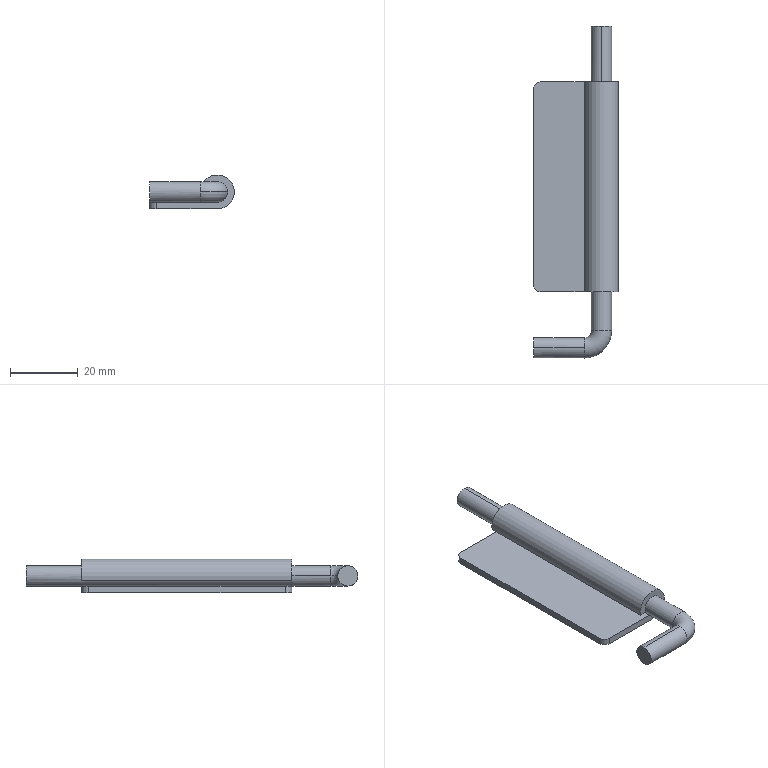Part | SolidWorks | features Extrusion 1, Fillet 1, Sweep 1 | 1 solid | 19 faces | box 25 x 98 x 10 mm | volume 8135 mm3 | cylinder 9 | plane 8 | torus 2 | commonest cylinder face diameters 6 x6 4 x2 10 x1
STEP:
#1=CARTESIAN_POINT('',(-5.,-19.5,0.));
#2=VERTEX_POINT('',#1);
#3=CARTESIAN_POINT('',(-5.,-16.5,3.));
#4=VERTEX_POINT('',#3);
#5=CARTESIAN_POINT('',(-5.,-16.5,0.));
#6=DIRECTION('',(-1.,0.,0.));
#7=DIRECTION('',(0.,0.,-1.));
#8=AXIS2_PLACEMENT_3D('',#5,#6,#7);
#9=CIRCLE('',#8,3.);
#10=EDGE_CURVE('',#2,#4,#9,.T.);
#11=ORIENTED_EDGE('',*,*,#10,.F.);
#12=CARTESIAN_POINT('',(3.,-11.5,0.));
#13=VERTEX_POINT('',#12);
#14=CARTESIAN_POINT('',(-5.,-11.5,0.));
#15=DIRECTION('',(0.,0.,1.));
#16=DIRECTION('',(1.,0.,0.));
#17=AXIS2_PLACEMENT_3D('',#14,#15,#16);
#18=CIRCLE('',#17,8.);
#19=EDGE_CURVE('',#2,#13,#18,.T.);
#20=ORIENTED_EDGE('',*,*,#19,.T.);
#21=CARTESIAN_POINT('',(-3.,-11.5,0.));
#22=VERTEX_POINT('',#21);
#23=CARTESIAN_POINT('',(0.,-11.5,0.));
#24=DIRECTION('',(0.,-1.,0.));
#25=DIRECTION('',(0.,0.,-1.));
#26=AXIS2_PLACEMENT_3D('',#23,#24,#25);
#27=CIRCLE('',#26,3.);
#28=EDGE_CURVE('',#13,#22,#27,.T.);
#29=ORIENTED_EDGE('',*,*,#28,.T.);
#30=CARTESIAN_POINT('',(-5.,-13.5,0.));
#31=VERTEX_POINT('',#30);
#32=CARTESIAN_POINT('',(-5.,-11.5,0.));
#33=DIRECTION('',(0.,0.,1.));
#34=DIRECTION('',(1.,0.,0.));
#35=AXIS2_PLACEMENT_3D('',#32,#33,#34);
#36=CIRCLE('',#35,2.);
#37=EDGE_CURVE('',#31,#22,#36,.T.);
#38=ORIENTED_EDGE('',*,*,#37,.F.);
#39=CARTESIAN_POINT('',(-5.,-16.5,0.));
#40=DIRECTION('',(-1.,0.,0.));
#41=DIRECTION('',(0.,0.,-1.));
#42=AXIS2_PLACEMENT_3D('',#39,#40,#41);
#43=CIRCLE('',#42,3.);
#44=EDGE_CURVE('',#4,#31,#43,.T.);
#45=ORIENTED_EDGE('',*,*,#44,.F.);
#46=EDGE_LOOP('',(#11,#20,#29,#38,#45));
#47=FACE_OUTER_BOUND('',#46,.T.);
#48=CARTESIAN_POINT('',(-5.,-11.5,0.));
#49=DIRECTION('',(0.,0.,1.));
#50=DIRECTION('',(1.,0.,0.));
#51=AXIS2_PLACEMENT_3D('',#48,#49,#50);
#52=TOROIDAL_SURFACE('',#51,5.,3.);
#53=ADVANCED_FACE('',(#47),#52,.T.);
#54=ORIENTED_EDGE('',*,*,#28,.F.);
#55=CARTESIAN_POINT('',(3.,0.,0.));
#56=VERTEX_POINT('',#55);
#57=CARTESIAN_POINT('',(3.,-11.5,0.));
#58=DIRECTION('',(0.,1.,0.));
#59=VECTOR('',#58,1000.);
#60=LINE('',#57,#59);
#61=EDGE_CURVE('',#13,#56,#60,.T.);
#62=ORIENTED_EDGE('',*,*,#61,.T.);
#63=CARTESIAN_POINT('',(-3.,0.,0.));
#64=VERTEX_POINT('',#63);
#65=CARTESIAN_POINT('',(0.,0.,0.));
#66=DIRECTION('',(0.,-1.,0.));
#67=DIRECTION('',(0.,0.,1.));
#68=AXIS2_PLACEMENT_3D('',#65,#66,#67);
#69=CIRCLE('',#68,3.);
#70=EDGE_CURVE('',#56,#64,#69,.T.);
#71=ORIENTED_EDGE('',*,*,#70,.T.);
#72=CARTESIAN_POINT('',(-3.,-11.5,0.));
#73=DIRECTION('',(0.,1.,0.));
#74=VECTOR('',#73,1000.);
#75=LINE('',#72,#74);
#76=EDGE_CURVE('',#22,#64,#75,.T.);
#77=ORIENTED_EDGE('',*,*,#76,.F.);
#78=EDGE_LOOP('',(#54,#62,#71,#77));
#79=FACE_OUTER_BOUND('',#78,.T.);
#80=CARTESIAN_POINT('',(0.,-11.5,0.));
#81=DIRECTION('',(0.,1.,0.));
#82=DIRECTION('',(-1.,0.,0.));
#83=AXIS2_PLACEMENT_3D('',#80,#81,#82);
#84=CYLINDRICAL_SURFACE('',#83,3.);
#85=ADVANCED_FACE('',(#79),#84,.T.);
#86=CARTESIAN_POINT('',(-20.,-16.5,3.));
#87=VERTEX_POINT('',#86);
#88=CARTESIAN_POINT('',(-20.,-16.5,-3.));
#89=VERTEX_POINT('',#88);
#90=CARTESIAN_POINT('',(-20.,-16.5,0.));
#91=DIRECTION('',(-1.,0.,0.));
#92=DIRECTION('',(0.,0.,-1.));
#93=AXIS2_PLACEMENT_3D('',#90,#91,#92);
#94=CIRCLE('',#93,3.);
#95=EDGE_CURVE('',#87,#89,#94,.T.);
#96=ORIENTED_EDGE('',*,*,#95,.F.);
#97=CARTESIAN_POINT('',(-20.,-16.5,3.));
#98=DIRECTION('',(1.,0.,0.));
#99=VECTOR('',#98,1000.);
#100=LINE('',#97,#99);
#101=EDGE_CURVE('',#87,#4,#100,.T.);
#102=ORIENTED_EDGE('',*,*,#101,.T.);
#103=ORIENTED_EDGE('',*,*,#44,.T.);
#104=CARTESIAN_POINT('',(-5.,-16.5,-3.));
#105=VERTEX_POINT('',#104);
#106=CARTESIAN_POINT('',(-5.,-16.5,0.));
#107=DIRECTION('',(-1.,0.,0.));
#108=DIRECTION('',(0.,0.,-1.));
#109=AXIS2_PLACEMENT_3D('',#106,#107,#108);
#110=CIRCLE('',#109,3.);
#111=EDGE_CURVE('',#31,#105,#110,.T.);
#112=ORIENTED_EDGE('',*,*,#111,.T.);
#113=CARTESIAN_POINT('',(-20.,-16.5,-3.));
#114=DIRECTION('',(1.,0.,0.));
#115=VECTOR('',#114,1000.);
#116=LINE('',#113,#115);
#117=EDGE_CURVE('',#89,#105,#116,.T.);
#118=ORIENTED_EDGE('',*,*,#117,.F.);
#119=EDGE_LOOP('',(#96,#102,#103,#112,#118));
#120=FACE_OUTER_BOUND('',#119,.T.);
#121=CARTESIAN_POINT('',(-20.,-16.5,0.));
#122=DIRECTION('',(1.,0.,0.));
#123=DIRECTION('',(0.,0.,-1.));
#124=AXIS2_PLACEMENT_3D('',#121,#122,#123);
#125=CYLINDRICAL_SURFACE('',#124,3.);
#126=ADVANCED_FACE('',(#120),#125,.T.);
#127=CARTESIAN_POINT('',(0.,62.,-3.));
#128=VERTEX_POINT('',#127);
#129=CARTESIAN_POINT('',(0.,62.,3.));
#130=VERTEX_POINT('',#129);
#131=CARTESIAN_POINT('',(0.,62.,0.));
#132=DIRECTION('',(0.,-1.,0.));
#133=DIRECTION('',(0.,0.,1.));
#134=AXIS2_PLACEMENT_3D('',#131,#132,#133);
#135=CIRCLE('',#134,3.);
#136=EDGE_CURVE('',#128,#130,#135,.T.);
#137=ORIENTED_EDGE('',*,*,#136,.F.);
#138=CARTESIAN_POINT('',(0.,78.5,-3.));
#139=VERTEX_POINT('',#138);
#140=CARTESIAN_POINT('',(0.,0.,-3.));
#141=DIRECTION('',(0.,1.,0.));
#142=VECTOR('',#141,1000.);
#143=LINE('',#140,#142);
#144=EDGE_CURVE('',#128,#139,#143,.T.);
#145=ORIENTED_EDGE('',*,*,#144,.T.);
#146=CARTESIAN_POINT('',(0.,78.5,3.));
#147=VERTEX_POINT('',#146);
#148=CARTESIAN_POINT('',(0.,78.5,0.));
#149=DIRECTION('',(0.,-1.,0.));
#150=DIRECTION('',(0.,0.,-1.));
#151=AXIS2_PLACEMENT_3D('',#148,#149,#150);
#152=CIRCLE('',#151,3.);
#153=EDGE_CURVE('',#139,#147,#152,.T.);
#154=ORIENTED_EDGE('',*,*,#153,.T.);
#155=CARTESIAN_POINT('',(0.,0.,3.));
#156=DIRECTION('',(0.,1.,0.));
#157=VECTOR('',#156,1000.);
#158=LINE('',#155,#157);
#159=EDGE_CURVE('',#130,#147,#158,.T.);
#160=ORIENTED_EDGE('',*,*,#159,.F.);
#161=EDGE_LOOP('',(#137,#145,#154,#160));
#162=FACE_OUTER_BOUND('',#161,.T.);
#163=CARTESIAN_POINT('',(0.,0.,0.));
#164=DIRECTION('',(0.,1.,0.));
#165=DIRECTION('',(0.,0.,1.));
#166=AXIS2_PLACEMENT_3D('',#163,#164,#165);
#167=CYLINDRICAL_SURFACE('',#166,3.);
#168=ADVANCED_FACE('',(#162),#167,.T.);
#169=CARTESIAN_POINT('',(-4.83,0.,-1.294));
#170=VERTEX_POINT('',#169);
#171=CARTESIAN_POINT('',(0.,0.,-5.));
#172=VERTEX_POINT('',#171);
#173=CARTESIAN_POINT('',(0.,0.,0.));
#174=DIRECTION('',(0.,1.,0.));
#175=DIRECTION('',(0.,0.,1.));
#176=AXIS2_PLACEMENT_3D('',#173,#174,#175);
#177=CIRCLE('',#176,5.);
#178=EDGE_CURVE('',#170,#172,#177,.T.);
#179=ORIENTED_EDGE('',*,*,#178,.T.);
#180=CARTESIAN_POINT('',(0.,62.,-5.));
#181=VERTEX_POINT('',#180);
#182=CARTESIAN_POINT('',(0.,62.,-5.));
#183=DIRECTION('',(0.,-1.,0.));
#184=VECTOR('',#183,1000.);
#185=LINE('',#182,#184);
#186=EDGE_CURVE('',#181,#172,#185,.T.);
#187=ORIENTED_EDGE('',*,*,#186,.F.);
#188=CARTESIAN_POINT('',(-4.83,62.,-1.294));
#189=VERTEX_POINT('',#188);
#190=CARTESIAN_POINT('',(0.,62.,0.));
#191=DIRECTION('',(0.,1.,0.));
#192=DIRECTION('',(0.,0.,1.));
#193=AXIS2_PLACEMENT_3D('',#190,#191,#192);
#194=CIRCLE('',#193,5.);
#195=EDGE_CURVE('',#189,#181,#194,.T.);
#196=ORIENTED_EDGE('',*,*,#195,.F.);
#197=CARTESIAN_POINT('',(-4.83,62.,-1.294));
#198=DIRECTION('',(0.,-1.,0.));
#199=VECTOR('',#198,1000.);
#200=LINE('',#197,#199);
#201=EDGE_CURVE('',#189,#170,#200,.T.);
#202=ORIENTED_EDGE('',*,*,#201,.T.);
#203=EDGE_LOOP('',(#179,#187,#196,#202));
#204=FACE_OUTER_BOUND('',#203,.T.);
#205=CARTESIAN_POINT('',(0.,62.,0.));
#206=DIRECTION('',(0.,-1.,0.));
#207=DIRECTION('',(0.,0.,-1.));
#208=AXIS2_PLACEMENT_3D('',#205,#206,#207);
#209=CYLINDRICAL_SURFACE('',#208,5.);
#210=ADVANCED_FACE('',(#204),#209,.T.);
#211=CARTESIAN_POINT('',(-18.,0.,-5.));
#212=VERTEX_POINT('',#211);
#213=CARTESIAN_POINT('',(0.,0.,-5.));
#214=DIRECTION('',(-1.,0.,0.));
#215=VECTOR('',#214,1000.);
#216=LINE('',#213,#215);
#217=EDGE_CURVE('',#172,#212,#216,.T.);
#218=ORIENTED_EDGE('',*,*,#217,.T.);
#219=CARTESIAN_POINT('',(-20.,2.,-5.));
#220=VERTEX_POINT('',#219);
#221=CARTESIAN_POINT('',(-18.,2.,-5.));
#222=DIRECTION('',(0.,0.,-1.));
#223=DIRECTION('',(1.,0.,0.));
#224=AXIS2_PLACEMENT_3D('',#221,#222,#223);
#225=CIRCLE('',#224,2.);
#226=EDGE_CURVE('',#212,#220,#225,.T.);
#227=ORIENTED_EDGE('',*,*,#226,.T.);
#228=CARTESIAN_POINT('',(-20.,60.,-5.));
#229=VERTEX_POINT('',#228);
#230=CARTESIAN_POINT('',(-20.,62.,-5.));
#231=DIRECTION('',(0.,-1.,0.));
#232=VECTOR('',#231,1000.);
#233=LINE('',#230,#232);
#234=EDGE_CURVE('',#229,#220,#233,.T.);
#235=ORIENTED_EDGE('',*,*,#234,.F.);
#236=CARTESIAN_POINT('',(-18.,62.,-5.));
#237=VERTEX_POINT('',#236);
#238=CARTESIAN_POINT('',(-18.,60.,-5.));
#239=DIRECTION('',(0.,0.,-1.));
#240=DIRECTION('',(1.,0.,0.));
#241=AXIS2_PLACEMENT_3D('',#238,#239,#240);
#242=CIRCLE('',#241,2.);
#243=EDGE_CURVE('',#229,#237,#242,.T.);
#244=ORIENTED_EDGE('',*,*,#243,.T.);
#245=CARTESIAN_POINT('',(0.,62.,-5.));
#246=DIRECTION('',(-1.,0.,0.));
#247=VECTOR('',#246,1000.);
#248=LINE('',#245,#247);
#249=EDGE_CURVE('',#181,#237,#248,.T.);
#250=ORIENTED_EDGE('',*,*,#249,.F.);
#251=ORIENTED_EDGE('',*,*,#186,.T.);
#252=EDGE_LOOP('',(#218,#227,#235,#244,#250,#251));
#253=FACE_OUTER_BOUND('',#252,.T.);
#254=CARTESIAN_POINT('',(0.,62.,-5.));
#255=DIRECTION('',(0.,0.,1.));
#256=DIRECTION('',(1.,0.,0.));
#257=AXIS2_PLACEMENT_3D('',#254,#255,#256);
#258=PLANE('',#257);
#259=ADVANCED_FACE('',(#253),#258,.F.);
#260=ORIENTED_EDGE('',*,*,#234,.T.);
#261=CARTESIAN_POINT('',(-20.,2.,-3.));
#262=VERTEX_POINT('',#261);
#263=CARTESIAN_POINT('',(-20.,2.,-3.));
#264=DIRECTION('',(0.,0.,1.));
#265=VECTOR('',#264,1000.);
#266=LINE('',#263,#265);
#267=EDGE_CURVE('',#220,#262,#266,.T.);
#268=ORIENTED_EDGE('',*,*,#267,.T.);
#269=CARTESIAN_POINT('',(-20.,60.,-3.));
#270=VERTEX_POINT('',#269);
#271=CARTESIAN_POINT('',(-20.,62.,-3.));
#272=DIRECTION('',(0.,-1.,0.));
#273=VECTOR('',#272,1000.);
#274=LINE('',#271,#273);
#275=EDGE_CURVE('',#270,#262,#274,.T.);
#276=ORIENTED_EDGE('',*,*,#275,.F.);
#277=CARTESIAN_POINT('',(-20.,60.,-5.));
#278=DIRECTION('',(0.,0.,-1.));
#279=VECTOR('',#278,1000.);
#280=LINE('',#277,#279);
#281=EDGE_CURVE('',#270,#229,#280,.T.);
#282=ORIENTED_EDGE('',*,*,#281,.T.);
#283=EDGE_LOOP('',(#260,#268,#276,#282));
#284=FACE_OUTER_BOUND('',#283,.T.);
#285=CARTESIAN_POINT('',(-20.,62.,-3.));
#286=DIRECTION('',(1.,0.,0.));
#287=DIRECTION('',(0.,0.,-1.));
#288=AXIS2_PLACEMENT_3D('',#285,#286,#287);
#289=PLANE('',#288);
#290=ADVANCED_FACE('',(#284),#289,.F.);
#291=ORIENTED_EDGE('',*,*,#275,.T.);
#292=CARTESIAN_POINT('',(-18.,0.,-3.));
#293=VERTEX_POINT('',#292);
#294=CARTESIAN_POINT('',(-18.,2.,-3.));
#295=DIRECTION('',(0.,0.,1.));
#296=DIRECTION('',(-1.,0.,0.));
#297=AXIS2_PLACEMENT_3D('',#294,#295,#296);
#298=CIRCLE('',#297,2.);
#299=EDGE_CURVE('',#262,#293,#298,.T.);
#300=ORIENTED_EDGE('',*,*,#299,.T.);
#301=CARTESIAN_POINT('',(0.,0.,-3.));
#302=VERTEX_POINT('',#301);
#303=CARTESIAN_POINT('',(0.,0.,-3.));
#304=DIRECTION('',(1.,0.,0.));
#305=VECTOR('',#304,1000.);
#306=LINE('',#303,#305);
#307=EDGE_CURVE('',#293,#302,#306,.T.);
#308=ORIENTED_EDGE('',*,*,#307,.T.);
#309=CARTESIAN_POINT('',(0.,62.,-3.));
#310=DIRECTION('',(0.,-1.,0.));
#311=VECTOR('',#310,1000.);
#312=LINE('',#309,#311);
#313=EDGE_CURVE('',#128,#302,#312,.T.);
#314=ORIENTED_EDGE('',*,*,#313,.F.);
#315=CARTESIAN_POINT('',(-18.,62.,-3.));
#316=VERTEX_POINT('',#315);
#317=CARTESIAN_POINT('',(0.,62.,-3.));
#318=DIRECTION('',(1.,0.,0.));
#319=VECTOR('',#318,1000.);
#320=LINE('',#317,#319);
#321=EDGE_CURVE('',#316,#128,#320,.T.);
#322=ORIENTED_EDGE('',*,*,#321,.F.);
#323=CARTESIAN_POINT('',(-18.,60.,-3.));
#324=DIRECTION('',(0.,0.,1.));
#325=DIRECTION('',(-1.,0.,0.));
#326=AXIS2_PLACEMENT_3D('',#323,#324,#325);
#327=CIRCLE('',#326,2.);
#328=EDGE_CURVE('',#316,#270,#327,.T.);
#329=ORIENTED_EDGE('',*,*,#328,.T.);
#330=EDGE_LOOP('',(#291,#300,#308,#314,#322,#329));
#331=FACE_OUTER_BOUND('',#330,.T.);
#332=CARTESIAN_POINT('',(0.,62.,-3.));
#333=DIRECTION('',(0.,0.,-1.));
#334=DIRECTION('',(-1.,0.,0.));
#335=AXIS2_PLACEMENT_3D('',#332,#333,#334);
#336=PLANE('',#335);
#337=ADVANCED_FACE('',(#331),#336,.F.);
#338=CARTESIAN_POINT('',(-2.898,0.,-0.7765));
#339=VERTEX_POINT('',#338);
#340=CARTESIAN_POINT('',(-4.83,0.,-1.294));
#341=DIRECTION('',(-0.9659,0.,-0.2588));
#342=VECTOR('',#341,1000.);
#343=LINE('',#340,#342);
#344=EDGE_CURVE('',#339,#170,#343,.T.);
#345=ORIENTED_EDGE('',*,*,#344,.T.);
#346=ORIENTED_EDGE('',*,*,#201,.F.);
#347=CARTESIAN_POINT('',(-2.898,62.,-0.7765));
#348=VERTEX_POINT('',#347);
#349=CARTESIAN_POINT('',(-4.83,62.,-1.294));
#350=DIRECTION('',(-0.9659,0.,-0.2588));
#351=VECTOR('',#350,1000.);
#352=LINE('',#349,#351);
#353=EDGE_CURVE('',#348,#189,#352,.T.);
#354=ORIENTED_EDGE('',*,*,#353,.F.);
#355=CARTESIAN_POINT('',(-2.898,62.,-0.7765));
#356=DIRECTION('',(0.,-1.,0.));
#357=VECTOR('',#356,1000.);
#358=LINE('',#355,#357);
#359=EDGE_CURVE('',#348,#339,#358,.T.);
#360=ORIENTED_EDGE('',*,*,#359,.T.);
#361=EDGE_LOOP('',(#345,#346,#354,#360));
#362=FACE_OUTER_BOUND('',#361,.T.);
#363=CARTESIAN_POINT('',(-4.83,62.,-1.294));
#364=DIRECTION('',(-0.2588,0.,0.9659));
#365=DIRECTION('',(0.9659,0.,0.2588));
#366=AXIS2_PLACEMENT_3D('',#363,#364,#365);
#367=PLANE('',#366);
#368=ADVANCED_FACE('',(#362),#367,.F.);
#369=ORIENTED_EDGE('',*,*,#249,.T.);
#370=CARTESIAN_POINT('',(-18.,62.,-3.));
#371=DIRECTION('',(0.,0.,1.));
#372=VECTOR('',#371,1000.);
#373=LINE('',#370,#372);
#374=EDGE_CURVE('',#237,#316,#373,.T.);
#375=ORIENTED_EDGE('',*,*,#374,.T.);
#376=ORIENTED_EDGE('',*,*,#321,.T.);
#377=ORIENTED_EDGE('',*,*,#136,.T.);
#378=CARTESIAN_POINT('',(0.,62.,0.));
#379=DIRECTION('',(0.,-1.,0.));
#380=DIRECTION('',(0.,0.,1.));
#381=AXIS2_PLACEMENT_3D('',#378,#379,#380);
#382=CIRCLE('',#381,3.);
#383=EDGE_CURVE('',#130,#348,#382,.T.);
#384=ORIENTED_EDGE('',*,*,#383,.T.);
#385=ORIENTED_EDGE('',*,*,#353,.T.);
#386=ORIENTED_EDGE('',*,*,#195,.T.);
#387=EDGE_LOOP('',(#369,#375,#376,#377,#384,#385,#386));
#388=FACE_OUTER_BOUND('',#387,.T.);
#389=CARTESIAN_POINT('',(0.,62.,0.));
#390=DIRECTION('',(0.,1.,0.));
#391=DIRECTION('',(0.,0.,1.));
#392=AXIS2_PLACEMENT_3D('',#389,#390,#391);
#393=PLANE('',#392);
#394=ADVANCED_FACE('',(#388),#393,.T.);
#395=ORIENTED_EDGE('',*,*,#307,.F.);
#396=CARTESIAN_POINT('',(-18.,0.,0.));
#397=DIRECTION('',(0.,0.,-1.));
#398=VECTOR('',#397,1000.);
#399=LINE('',#396,#398);
#400=EDGE_CURVE('',#293,#212,#399,.T.);
#401=ORIENTED_EDGE('',*,*,#400,.T.);
#402=ORIENTED_EDGE('',*,*,#217,.F.);
#403=ORIENTED_EDGE('',*,*,#178,.F.);
#404=ORIENTED_EDGE('',*,*,#344,.F.);
#405=CARTESIAN_POINT('',(0.,0.,0.));
#406=DIRECTION('',(0.,-1.,0.));
#407=DIRECTION('',(0.,0.,1.));
#408=AXIS2_PLACEMENT_3D('',#405,#406,#407);
#409=CIRCLE('',#408,3.);
#410=EDGE_CURVE('',#64,#339,#409,.T.);
#411=ORIENTED_EDGE('',*,*,#410,.F.);
#412=ORIENTED_EDGE('',*,*,#70,.F.);
#413=CARTESIAN_POINT('',(0.,0.,0.));
#414=DIRECTION('',(0.,-1.,0.));
#415=DIRECTION('',(0.,0.,1.));
#416=AXIS2_PLACEMENT_3D('',#413,#414,#415);
#417=CIRCLE('',#416,3.);
#418=EDGE_CURVE('',#302,#56,#417,.T.);
#419=ORIENTED_EDGE('',*,*,#418,.F.);
#420=EDGE_LOOP('',(#395,#401,#402,#403,#404,#411,#412,#419));
#421=FACE_OUTER_BOUND('',#420,.T.);
#422=CARTESIAN_POINT('',(0.,0.,0.));
#423=DIRECTION('',(0.,1.,0.));
#424=DIRECTION('',(0.,0.,1.));
#425=AXIS2_PLACEMENT_3D('',#422,#423,#424);
#426=PLANE('',#425);
#427=ADVANCED_FACE('',(#421),#426,.F.);
#428=ORIENTED_EDGE('',*,*,#144,.F.);
#429=ORIENTED_EDGE('',*,*,#313,.T.);
#430=CARTESIAN_POINT('',(0.,0.,0.));
#431=DIRECTION('',(0.,-1.,0.));
#432=DIRECTION('',(0.,0.,-1.));
#433=AXIS2_PLACEMENT_3D('',#430,#431,#432);
#434=CIRCLE('',#433,3.);
#435=EDGE_CURVE('',#339,#302,#434,.T.);
#436=ORIENTED_EDGE('',*,*,#435,.F.);
#437=ORIENTED_EDGE('',*,*,#359,.F.);
#438=ORIENTED_EDGE('',*,*,#383,.F.);
#439=ORIENTED_EDGE('',*,*,#159,.T.);
#440=CARTESIAN_POINT('',(0.,78.5,0.));
#441=DIRECTION('',(0.,-1.,0.));
#442=DIRECTION('',(0.,0.,-1.));
#443=AXIS2_PLACEMENT_3D('',#440,#441,#442);
#444=CIRCLE('',#443,3.);
#445=EDGE_CURVE('',#147,#139,#444,.T.);
#446=ORIENTED_EDGE('',*,*,#445,.T.);
#447=EDGE_LOOP('',(#428,#429,#436,#437,#438,#439,#446));
#448=FACE_OUTER_BOUND('',#447,.T.);
#449=CARTESIAN_POINT('',(0.,0.,0.));
#450=DIRECTION('',(0.,1.,0.));
#451=DIRECTION('',(0.,0.,1.));
#452=AXIS2_PLACEMENT_3D('',#449,#450,#451);
#453=CYLINDRICAL_SURFACE('',#452,3.);
#454=ADVANCED_FACE('',(#448),#453,.T.);
#455=ORIENTED_EDGE('',*,*,#61,.F.);
#456=CARTESIAN_POINT('',(0.,-11.5,0.));
#457=DIRECTION('',(0.,-1.,0.));
#458=DIRECTION('',(0.,0.,-1.));
#459=AXIS2_PLACEMENT_3D('',#456,#457,#458);
#460=CIRCLE('',#459,3.);
#461=EDGE_CURVE('',#22,#13,#460,.T.);
#462=ORIENTED_EDGE('',*,*,#461,.F.);
#463=ORIENTED_EDGE('',*,*,#76,.T.);
#464=ORIENTED_EDGE('',*,*,#410,.T.);
#465=ORIENTED_EDGE('',*,*,#435,.T.);
#466=ORIENTED_EDGE('',*,*,#418,.T.);
#467=EDGE_LOOP('',(#455,#462,#463,#464,#465,#466));
#468=FACE_OUTER_BOUND('',#467,.T.);
#469=CARTESIAN_POINT('',(0.,-11.5,0.));
#470=DIRECTION('',(0.,1.,0.));
#471=DIRECTION('',(-1.,0.,0.));
#472=AXIS2_PLACEMENT_3D('',#469,#470,#471);
#473=CYLINDRICAL_SURFACE('',#472,3.);
#474=ADVANCED_FACE('',(#468),#473,.T.);
#475=ORIENTED_EDGE('',*,*,#19,.F.);
#476=CARTESIAN_POINT('',(-5.,-16.5,0.));
#477=DIRECTION('',(-1.,0.,0.));
#478=DIRECTION('',(0.,0.,-1.));
#479=AXIS2_PLACEMENT_3D('',#476,#477,#478);
#480=CIRCLE('',#479,3.);
#481=EDGE_CURVE('',#105,#2,#480,.T.);
#482=ORIENTED_EDGE('',*,*,#481,.F.);
#483=ORIENTED_EDGE('',*,*,#111,.F.);
#484=ORIENTED_EDGE('',*,*,#37,.T.);
#485=ORIENTED_EDGE('',*,*,#461,.T.);
#486=EDGE_LOOP('',(#475,#482,#483,#484,#485));
#487=FACE_OUTER_BOUND('',#486,.T.);
#488=CARTESIAN_POINT('',(-5.,-11.5,0.));
#489=DIRECTION('',(0.,0.,1.));
#490=DIRECTION('',(1.,0.,0.));
#491=AXIS2_PLACEMENT_3D('',#488,#489,#490);
#492=TOROIDAL_SURFACE('',#491,5.,3.);
#493=ADVANCED_FACE('',(#487),#492,.T.);
#494=ORIENTED_EDGE('',*,*,#101,.F.);
#495=CARTESIAN_POINT('',(-20.,-16.5,0.));
#496=DIRECTION('',(-1.,0.,0.));
#497=DIRECTION('',(0.,0.,-1.));
#498=AXIS2_PLACEMENT_3D('',#495,#496,#497);
#499=CIRCLE('',#498,3.);
#500=EDGE_CURVE('',#89,#87,#499,.T.);
#501=ORIENTED_EDGE('',*,*,#500,.F.);
#502=ORIENTED_EDGE('',*,*,#117,.T.);
#503=ORIENTED_EDGE('',*,*,#481,.T.);
#504=ORIENTED_EDGE('',*,*,#10,.T.);
#505=EDGE_LOOP('',(#494,#501,#502,#503,#504));
#506=FACE_OUTER_BOUND('',#505,.T.);
#507=CARTESIAN_POINT('',(-20.,-16.5,0.));
#508=DIRECTION('',(1.,0.,0.));
#509=DIRECTION('',(0.,0.,-1.));
#510=AXIS2_PLACEMENT_3D('',#507,#508,#509);
#511=CYLINDRICAL_SURFACE('',#510,3.);
#512=ADVANCED_FACE('',(#506),#511,.T.);
#513=ORIENTED_EDGE('',*,*,#445,.F.);
#514=ORIENTED_EDGE('',*,*,#153,.F.);
#515=EDGE_LOOP('',(#513,#514));
#516=FACE_OUTER_BOUND('',#515,.T.);
#517=CARTESIAN_POINT('',(0.,78.5,0.));
#518=DIRECTION('',(0.,-1.,0.));
#519=DIRECTION('',(0.,0.,-1.));
#520=AXIS2_PLACEMENT_3D('',#517,#518,#519);
#521=PLANE('',#520);
#522=ADVANCED_FACE('',(#516),#521,.F.);
#523=ORIENTED_EDGE('',*,*,#500,.T.);
#524=ORIENTED_EDGE('',*,*,#95,.T.);
#525=EDGE_LOOP('',(#523,#524));
#526=FACE_OUTER_BOUND('',#525,.T.);
#527=CARTESIAN_POINT('',(-20.,-16.5,0.));
#528=DIRECTION('',(-1.,0.,0.));
#529=DIRECTION('',(0.,0.,-1.));
#530=AXIS2_PLACEMENT_3D('',#527,#528,#529);
#531=PLANE('',#530);
#532=ADVANCED_FACE('',(#526),#531,.T.);
#533=ORIENTED_EDGE('',*,*,#226,.F.);
#534=ORIENTED_EDGE('',*,*,#400,.F.);
#535=ORIENTED_EDGE('',*,*,#299,.F.);
#536=ORIENTED_EDGE('',*,*,#267,.F.);
#537=EDGE_LOOP('',(#533,#534,#535,#536));
#538=FACE_OUTER_BOUND('',#537,.T.);
#539=CARTESIAN_POINT('',(-18.,2.,-3.));
#540=DIRECTION('',(0.,0.,1.));
#541=DIRECTION('',(1.,0.,0.));
#542=AXIS2_PLACEMENT_3D('',#539,#540,#541);
#543=CYLINDRICAL_SURFACE('',#542,2.);
#544=ADVANCED_FACE('',(#538),#543,.T.);
#545=ORIENTED_EDGE('',*,*,#243,.F.);
#546=ORIENTED_EDGE('',*,*,#281,.F.);
#547=ORIENTED_EDGE('',*,*,#328,.F.);
#548=ORIENTED_EDGE('',*,*,#374,.F.);
#549=EDGE_LOOP('',(#545,#546,#547,#548));
#550=FACE_OUTER_BOUND('',#549,.T.);
#551=CARTESIAN_POINT('',(-18.,60.,0.));
#552=DIRECTION('',(0.,0.,-1.));
#553=DIRECTION('',(-1.,0.,0.));
#554=AXIS2_PLACEMENT_3D('',#551,#552,#553);
#555=CYLINDRICAL_SURFACE('',#554,2.);
#556=ADVANCED_FACE('',(#550),#555,.T.);
#557=CLOSED_SHELL('',(#53,#85,#126,#168,#210,#259,#290,#337,#368,#394,#427,#454,#474,#493,#512,#522,#532,#544,#556));
#558=MANIFOLD_SOLID_BREP('',#557);
#559=CARTESIAN_POINT('',(0.,0.,0.));
#560=DIRECTION('',(0.,0.,1.));
#561=DIRECTION('',(1.,0.,0.));
#562=AXIS2_PLACEMENT_3D('',#559,#560,#561);
#563=(LENGTH_UNIT()NAMED_UNIT(*)SI_UNIT(.MILLI.,.METRE.));
#564=UNCERTAINTY_MEASURE_WITH_UNIT(LENGTH_MEASURE(0.00001),#563,'','');
#565=(NAMED_UNIT(*)PLANE_ANGLE_UNIT()SI_UNIT($,.RADIAN.));
#566=(NAMED_UNIT(*)SI_UNIT($,.STERADIAN.)SOLID_ANGLE_UNIT());
#567=(GEOMETRIC_REPRESENTATION_CONTEXT(3)GLOBAL_UNCERTAINTY_ASSIGNED_CONTEXT((#564))GLOBAL_UNIT_ASSIGNED_CONTEXT((#563,#565,#566))REPRESENTATION_CONTEXT('',''));
#568=ADVANCED_BREP_SHAPE_REPRESENTATION('',(#558,#562),#567);